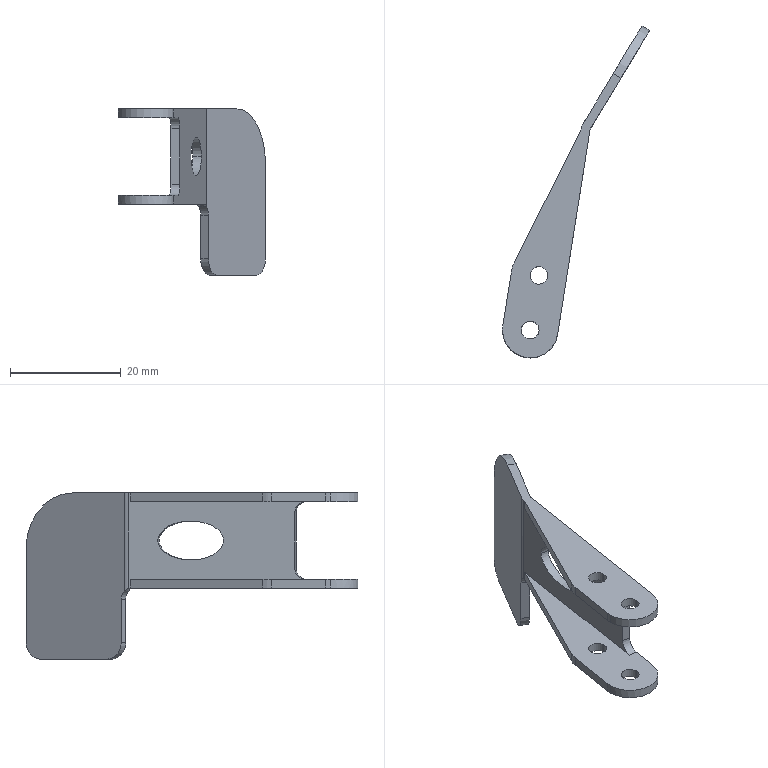Part | SolidWorks | features BaseBody 1 | 1 solid | 42 faces | box 26.504 x 59.832 x 30 mm | volume 2438 mm3 | cylinder 23 | plane 16 | spline 3 | commonest cylinder face diameters 3.2 x8 10 x6 4 x4 6 x2 1.117 x1 4.317 x1